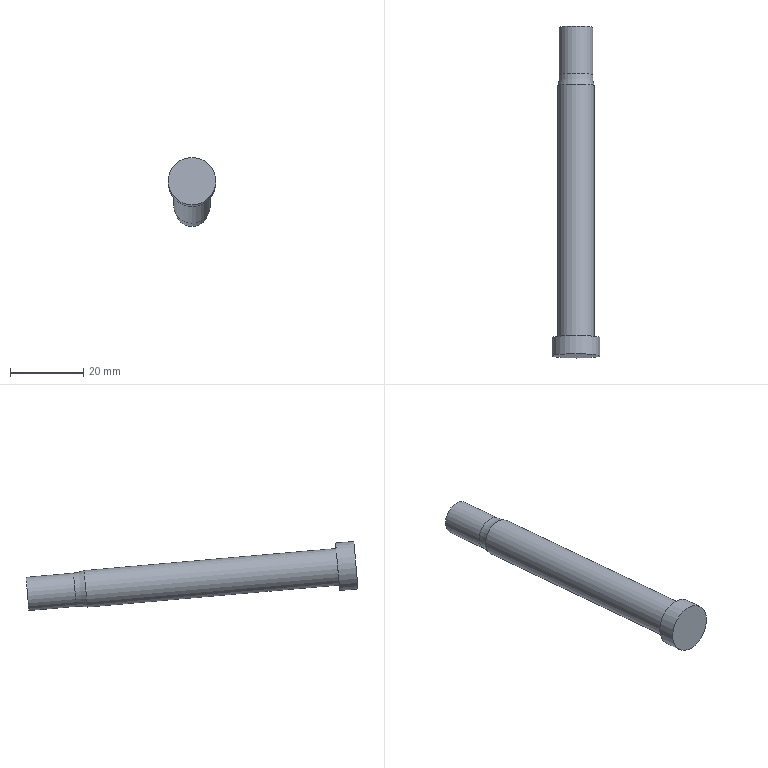Part | NX | features SPAS 10-80-9.100 2 | 1 solid | 7 faces | box 13 x 90.621 x 18.852 mm | volume 7137 mm3 | plane 3 | cylinder 3 | torus 1 | commonest cylinder face diameters 9.1 x1 10 x1 13 x1
STEP:
#1=CARTESIAN_POINT('',(280.775,-55.774,-54.63));
#2=VERTEX_POINT('',#1);
#3=CARTESIAN_POINT('',(280.775,-55.377,-50.098));
#4=DIRECTION('',(0.,-0.9962,0.08716));
#5=DIRECTION('',(0.,-0.08716,-0.9962));
#6=AXIS2_PLACEMENT_3D('',#3,#4,#5);
#7=CIRCLE('',#6,4.55);
#8=EDGE_CURVE('',#2,#2,#7,.T.);
#9=ORIENTED_EDGE('',*,*,#8,.F.);
#10=EDGE_LOOP('',(#9));
#11=FACE_BOUND('',#10,.T.);
#12=CARTESIAN_POINT('',(280.775,-55.377,-50.098));
#13=DIRECTION('',(0.,0.9962,-0.08716));
#14=DIRECTION('',(0.,0.08716,0.9962));
#15=AXIS2_PLACEMENT_3D('',#12,#13,#14);
#16=PLANE('',#15);
#17=ADVANCED_FACE('',(#11),#16,.T.);
#18=CARTESIAN_POINT('',(280.775,-68.724,-53.497));
#19=VERTEX_POINT('',#18);
#20=CARTESIAN_POINT('',(280.775,-68.328,-48.965));
#21=DIRECTION('',(0.,-0.9962,0.08716));
#22=DIRECTION('',(0.,-0.08716,-0.9962));
#23=AXIS2_PLACEMENT_3D('',#20,#21,#22);
#24=CIRCLE('',#23,4.55);
#25=EDGE_CURVE('',#19,#19,#24,.F.);
#26=ORIENTED_EDGE('',*,*,#25,.T.);
#27=EDGE_LOOP('',(#26));
#28=FACE_BOUND('',#27,.T.);
#29=ORIENTED_EDGE('',*,*,#8,.T.);
#30=EDGE_LOOP('',(#29));
#31=FACE_BOUND('',#30,.T.);
#32=CARTESIAN_POINT('',(280.775,-55.377,-50.098));
#33=DIRECTION('',(0.,-0.9962,0.08716));
#34=DIRECTION('',(0.,-0.08716,-0.9962));
#35=AXIS2_PLACEMENT_3D('',#32,#33,#34);
#36=CYLINDRICAL_SURFACE('',#35,4.55);
#37=ADVANCED_FACE('',(#28,#31),#36,.T.);
#38=CARTESIAN_POINT('',(280.775,-139.618,-37.709));
#39=VERTEX_POINT('',#38);
#40=CARTESIAN_POINT('',(280.775,-140.054,-42.689));
#41=DIRECTION('',(0.,0.9962,-0.08716));
#42=DIRECTION('',(0.,0.08716,0.9962));
#43=AXIS2_PLACEMENT_3D('',#40,#41,#42);
#44=CIRCLE('',#43,5.);
#45=EDGE_CURVE('',#39,#39,#44,.F.);
#46=ORIENTED_EDGE('',*,*,#45,.F.);
#47=EDGE_LOOP('',(#46));
#48=FACE_BOUND('',#47,.T.);
#49=CARTESIAN_POINT('',(280.775,-71.718,-53.687));
#50=VERTEX_POINT('',#49);
#51=CARTESIAN_POINT('',(280.775,-71.283,-48.706));
#52=DIRECTION('',(0.,-0.9962,0.08716));
#53=DIRECTION('',(0.,-0.08716,-0.9962));
#54=AXIS2_PLACEMENT_3D('',#51,#52,#53);
#55=CIRCLE('',#54,5.);
#56=EDGE_CURVE('',#50,#50,#55,.T.);
#57=ORIENTED_EDGE('',*,*,#56,.T.);
#58=EDGE_LOOP('',(#57));
#59=FACE_BOUND('',#58,.T.);
#60=CARTESIAN_POINT('',(280.775,-71.283,-48.706));
#61=DIRECTION('',(0.,-0.9962,0.08716));
#62=DIRECTION('',(0.,-0.08716,-0.9962));
#63=AXIS2_PLACEMENT_3D('',#60,#61,#62);
#64=CYLINDRICAL_SURFACE('',#63,5.);
#65=ADVANCED_FACE('',(#48,#59),#64,.T.);
#66=CARTESIAN_POINT('',(280.775,-145.601,-48.729));
#67=VERTEX_POINT('',#66);
#68=CARTESIAN_POINT('',(280.775,-145.035,-42.254));
#69=DIRECTION('',(0.,-0.9962,0.08716));
#70=DIRECTION('',(0.,-0.08716,-0.9962));
#71=AXIS2_PLACEMENT_3D('',#68,#69,#70);
#72=CIRCLE('',#71,6.5);
#73=EDGE_CURVE('',#67,#67,#72,.F.);
#74=ORIENTED_EDGE('',*,*,#73,.F.);
#75=EDGE_LOOP('',(#74));
#76=FACE_BOUND('',#75,.T.);
#77=CARTESIAN_POINT('',(280.775,-145.035,-42.254));
#78=DIRECTION('',(0.,-0.9962,0.08716));
#79=DIRECTION('',(0.,-0.08716,-0.9962));
#80=AXIS2_PLACEMENT_3D('',#77,#78,#79);
#81=PLANE('',#80);
#82=ADVANCED_FACE('',(#76),#81,.T.);
#83=ORIENTED_EDGE('',*,*,#45,.T.);
#84=EDGE_LOOP('',(#83));
#85=FACE_BOUND('',#84,.T.);
#86=CARTESIAN_POINT('',(280.775,-139.487,-36.214));
#87=VERTEX_POINT('',#86);
#88=CARTESIAN_POINT('',(280.775,-140.054,-42.689));
#89=DIRECTION('',(0.,0.9962,-0.08716));
#90=DIRECTION('',(0.,0.08716,0.9962));
#91=AXIS2_PLACEMENT_3D('',#88,#89,#90);
#92=CIRCLE('',#91,6.5);
#93=EDGE_CURVE('',#87,#87,#92,.F.);
#94=ORIENTED_EDGE('',*,*,#93,.F.);
#95=EDGE_LOOP('',(#94));
#96=FACE_BOUND('',#95,.T.);
#97=CARTESIAN_POINT('',(280.775,-140.054,-42.689));
#98=DIRECTION('',(0.,0.9962,-0.08716));
#99=DIRECTION('',(0.,0.08716,0.9962));
#100=AXIS2_PLACEMENT_3D('',#97,#98,#99);
#101=PLANE('',#100);
#102=ADVANCED_FACE('',(#85,#96),#101,.T.);
#103=ORIENTED_EDGE('',*,*,#73,.T.);
#104=EDGE_LOOP('',(#103));
#105=FACE_BOUND('',#104,.T.);
#106=ORIENTED_EDGE('',*,*,#93,.T.);
#107=EDGE_LOOP('',(#106));
#108=FACE_BOUND('',#107,.T.);
#109=CARTESIAN_POINT('',(280.775,-130.092,-43.561));
#110=DIRECTION('',(0.,-0.9962,0.08716));
#111=DIRECTION('',(0.,-0.08716,-0.9962));
#112=AXIS2_PLACEMENT_3D('',#109,#110,#111);
#113=CYLINDRICAL_SURFACE('',#112,6.5);
#114=ADVANCED_FACE('',(#105,#108),#113,.T.);
#115=ORIENTED_EDGE('',*,*,#25,.F.);
#116=EDGE_LOOP('',(#115));
#117=FACE_BOUND('',#116,.T.);
#118=ORIENTED_EDGE('',*,*,#56,.F.);
#119=EDGE_LOOP('',(#118));
#120=FACE_BOUND('',#119,.T.);
#121=CARTESIAN_POINT('',(280.775,-68.328,-48.965));
#122=DIRECTION('',(0.,-0.9962,0.08716));
#123=DIRECTION('',(0.,-0.08716,-0.9962));
#124=AXIS2_PLACEMENT_3D('',#121,#122,#123);
#125=TOROIDAL_SURFACE('',#124,14.55,10.);
#126=ADVANCED_FACE('',(#117,#120),#125,.F.);
#127=CLOSED_SHELL('',(#17,#37,#65,#82,#102,#114,#126));
#128=MANIFOLD_SOLID_BREP('',#127);
#129=(LENGTH_UNIT()NAMED_UNIT(*)SI_UNIT(.MILLI.,.METRE.));
#130=UNCERTAINTY_MEASURE_WITH_UNIT(LENGTH_MEASURE(0.00001),#129,'','');
#131=(NAMED_UNIT(*)PLANE_ANGLE_UNIT()SI_UNIT($,.RADIAN.));
#132=(NAMED_UNIT(*)SI_UNIT($,.STERADIAN.)SOLID_ANGLE_UNIT());
#133=(GEOMETRIC_REPRESENTATION_CONTEXT(3)GLOBAL_UNCERTAINTY_ASSIGNED_CONTEXT((#130))GLOBAL_UNIT_ASSIGNED_CONTEXT((#129,#131,#132))REPRESENTATION_CONTEXT('',''));
#134=ADVANCED_BREP_SHAPE_REPRESENTATION('',(#128),#133);